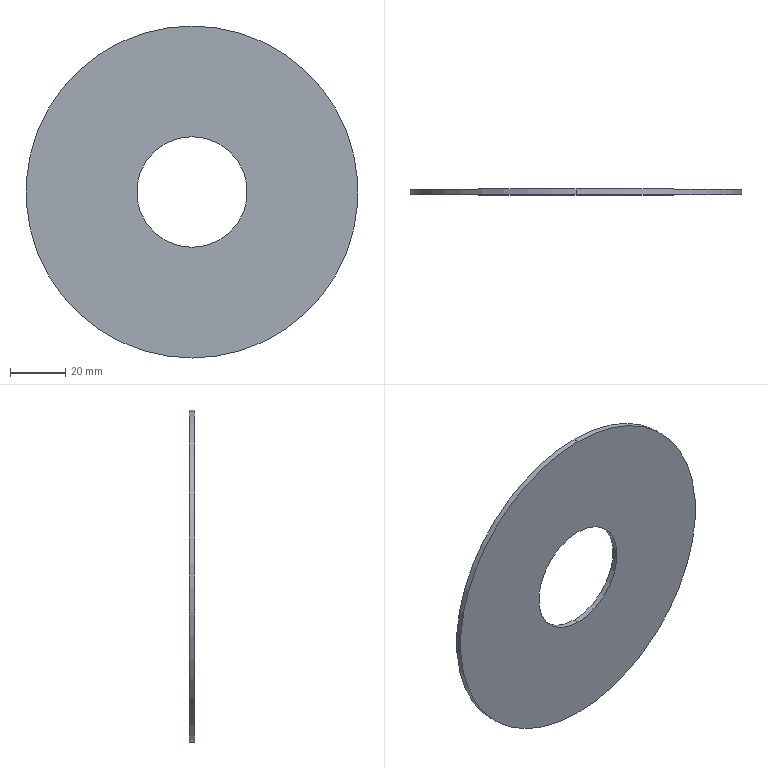Part | SolidWorks | features Extrusion 1 | 1 solid | 6 faces | box 120 x 2 x 120 mm | volume 20106 mm3 | cylinder 4 | plane 2 | commonest cylinder face diameters 40 x2 120 x2
STEP:
#1=CARTESIAN_POINT('',(0.,2.,-20.));
#2=VERTEX_POINT('',#1);
#3=CARTESIAN_POINT('',(0.,2.,20.));
#4=VERTEX_POINT('',#3);
#5=CARTESIAN_POINT('',(0.,2.,0.));
#6=DIRECTION('',(0.,1.,0.));
#7=DIRECTION('',(0.,0.,1.));
#8=AXIS2_PLACEMENT_3D('',#5,#6,#7);
#9=CIRCLE('',#8,20.);
#10=EDGE_CURVE('',#2,#4,#9,.T.);
#11=ORIENTED_EDGE('',*,*,#10,.T.);
#12=CARTESIAN_POINT('',(0.,0.,20.));
#13=VERTEX_POINT('',#12);
#14=CARTESIAN_POINT('',(0.,2.,20.));
#15=DIRECTION('',(0.,-1.,0.));
#16=VECTOR('',#15,1000.);
#17=LINE('',#14,#16);
#18=EDGE_CURVE('',#4,#13,#17,.T.);
#19=ORIENTED_EDGE('',*,*,#18,.T.);
#20=CARTESIAN_POINT('',(0.,0.,-20.));
#21=VERTEX_POINT('',#20);
#22=CARTESIAN_POINT('',(0.,0.,0.));
#23=DIRECTION('',(0.,1.,0.));
#24=DIRECTION('',(0.,0.,1.));
#25=AXIS2_PLACEMENT_3D('',#22,#23,#24);
#26=CIRCLE('',#25,20.);
#27=EDGE_CURVE('',#21,#13,#26,.T.);
#28=ORIENTED_EDGE('',*,*,#27,.F.);
#29=CARTESIAN_POINT('',(0.,2.,-20.));
#30=DIRECTION('',(0.,-1.,0.));
#31=VECTOR('',#30,1000.);
#32=LINE('',#29,#31);
#33=EDGE_CURVE('',#2,#21,#32,.T.);
#34=ORIENTED_EDGE('',*,*,#33,.F.);
#35=EDGE_LOOP('',(#11,#19,#28,#34));
#36=FACE_OUTER_BOUND('',#35,.T.);
#37=CARTESIAN_POINT('',(0.,2.,0.));
#38=DIRECTION('',(0.,-1.,0.));
#39=DIRECTION('',(0.,0.,-1.));
#40=AXIS2_PLACEMENT_3D('',#37,#38,#39);
#41=CYLINDRICAL_SURFACE('',#40,20.);
#42=ADVANCED_FACE('',(#36),#41,.F.);
#43=CARTESIAN_POINT('',(0.,2.,60.));
#44=VERTEX_POINT('',#43);
#45=CARTESIAN_POINT('',(0.,2.,-60.));
#46=VERTEX_POINT('',#45);
#47=CARTESIAN_POINT('',(0.,2.,0.));
#48=DIRECTION('',(0.,1.,0.));
#49=DIRECTION('',(0.,0.,1.));
#50=AXIS2_PLACEMENT_3D('',#47,#48,#49);
#51=CIRCLE('',#50,60.);
#52=EDGE_CURVE('',#44,#46,#51,.T.);
#53=ORIENTED_EDGE('',*,*,#52,.F.);
#54=CARTESIAN_POINT('',(0.,0.,60.));
#55=VERTEX_POINT('',#54);
#56=CARTESIAN_POINT('',(0.,2.,60.));
#57=DIRECTION('',(0.,-1.,0.));
#58=VECTOR('',#57,1000.);
#59=LINE('',#56,#58);
#60=EDGE_CURVE('',#44,#55,#59,.T.);
#61=ORIENTED_EDGE('',*,*,#60,.T.);
#62=CARTESIAN_POINT('',(0.,0.,-60.));
#63=VERTEX_POINT('',#62);
#64=CARTESIAN_POINT('',(0.,0.,0.));
#65=DIRECTION('',(0.,1.,0.));
#66=DIRECTION('',(0.,0.,1.));
#67=AXIS2_PLACEMENT_3D('',#64,#65,#66);
#68=CIRCLE('',#67,60.);
#69=EDGE_CURVE('',#55,#63,#68,.T.);
#70=ORIENTED_EDGE('',*,*,#69,.T.);
#71=CARTESIAN_POINT('',(0.,2.,-60.));
#72=DIRECTION('',(0.,-1.,0.));
#73=VECTOR('',#72,1000.);
#74=LINE('',#71,#73);
#75=EDGE_CURVE('',#46,#63,#74,.T.);
#76=ORIENTED_EDGE('',*,*,#75,.F.);
#77=EDGE_LOOP('',(#53,#61,#70,#76));
#78=FACE_OUTER_BOUND('',#77,.T.);
#79=CARTESIAN_POINT('',(0.,2.,0.));
#80=DIRECTION('',(0.,-1.,0.));
#81=DIRECTION('',(0.,0.,-1.));
#82=AXIS2_PLACEMENT_3D('',#79,#80,#81);
#83=CYLINDRICAL_SURFACE('',#82,60.);
#84=ADVANCED_FACE('',(#78),#83,.T.);
#85=CARTESIAN_POINT('',(0.,2.,0.));
#86=DIRECTION('',(0.,1.,0.));
#87=DIRECTION('',(0.,0.,1.));
#88=AXIS2_PLACEMENT_3D('',#85,#86,#87);
#89=CIRCLE('',#88,60.);
#90=EDGE_CURVE('',#46,#44,#89,.T.);
#91=ORIENTED_EDGE('',*,*,#90,.T.);
#92=ORIENTED_EDGE('',*,*,#52,.T.);
#93=EDGE_LOOP('',(#91,#92));
#94=FACE_OUTER_BOUND('',#93,.T.);
#95=ORIENTED_EDGE('',*,*,#10,.F.);
#96=CARTESIAN_POINT('',(0.,2.,0.));
#97=DIRECTION('',(0.,1.,0.));
#98=DIRECTION('',(0.,0.,1.));
#99=AXIS2_PLACEMENT_3D('',#96,#97,#98);
#100=CIRCLE('',#99,20.);
#101=EDGE_CURVE('',#4,#2,#100,.T.);
#102=ORIENTED_EDGE('',*,*,#101,.F.);
#103=EDGE_LOOP('',(#95,#102));
#104=FACE_BOUND('',#103,.T.);
#105=CARTESIAN_POINT('',(0.,2.,0.));
#106=DIRECTION('',(0.,1.,0.));
#107=DIRECTION('',(0.,0.,1.));
#108=AXIS2_PLACEMENT_3D('',#105,#106,#107);
#109=PLANE('',#108);
#110=ADVANCED_FACE('',(#94,#104),#109,.T.);
#111=CARTESIAN_POINT('',(0.,0.,0.));
#112=DIRECTION('',(0.,1.,0.));
#113=DIRECTION('',(0.,0.,1.));
#114=AXIS2_PLACEMENT_3D('',#111,#112,#113);
#115=CIRCLE('',#114,60.);
#116=EDGE_CURVE('',#63,#55,#115,.T.);
#117=ORIENTED_EDGE('',*,*,#116,.F.);
#118=ORIENTED_EDGE('',*,*,#69,.F.);
#119=EDGE_LOOP('',(#117,#118));
#120=FACE_OUTER_BOUND('',#119,.T.);
#121=ORIENTED_EDGE('',*,*,#27,.T.);
#122=CARTESIAN_POINT('',(0.,0.,0.));
#123=DIRECTION('',(0.,1.,0.));
#124=DIRECTION('',(0.,0.,1.));
#125=AXIS2_PLACEMENT_3D('',#122,#123,#124);
#126=CIRCLE('',#125,20.);
#127=EDGE_CURVE('',#13,#21,#126,.T.);
#128=ORIENTED_EDGE('',*,*,#127,.T.);
#129=EDGE_LOOP('',(#121,#128));
#130=FACE_BOUND('',#129,.T.);
#131=CARTESIAN_POINT('',(0.,0.,0.));
#132=DIRECTION('',(0.,1.,0.));
#133=DIRECTION('',(0.,0.,1.));
#134=AXIS2_PLACEMENT_3D('',#131,#132,#133);
#135=PLANE('',#134);
#136=ADVANCED_FACE('',(#120,#130),#135,.F.);
#137=ORIENTED_EDGE('',*,*,#60,.F.);
#138=ORIENTED_EDGE('',*,*,#90,.F.);
#139=ORIENTED_EDGE('',*,*,#75,.T.);
#140=ORIENTED_EDGE('',*,*,#116,.T.);
#141=EDGE_LOOP('',(#137,#138,#139,#140));
#142=FACE_OUTER_BOUND('',#141,.T.);
#143=CARTESIAN_POINT('',(0.,2.,0.));
#144=DIRECTION('',(0.,-1.,0.));
#145=DIRECTION('',(0.,0.,-1.));
#146=AXIS2_PLACEMENT_3D('',#143,#144,#145);
#147=CYLINDRICAL_SURFACE('',#146,60.);
#148=ADVANCED_FACE('',(#142),#147,.T.);
#149=ORIENTED_EDGE('',*,*,#18,.F.);
#150=ORIENTED_EDGE('',*,*,#101,.T.);
#151=ORIENTED_EDGE('',*,*,#33,.T.);
#152=ORIENTED_EDGE('',*,*,#127,.F.);
#153=EDGE_LOOP('',(#149,#150,#151,#152));
#154=FACE_OUTER_BOUND('',#153,.T.);
#155=CARTESIAN_POINT('',(0.,2.,0.));
#156=DIRECTION('',(0.,-1.,0.));
#157=DIRECTION('',(0.,0.,-1.));
#158=AXIS2_PLACEMENT_3D('',#155,#156,#157);
#159=CYLINDRICAL_SURFACE('',#158,20.);
#160=ADVANCED_FACE('',(#154),#159,.F.);
#161=CLOSED_SHELL('',(#42,#84,#110,#136,#148,#160));
#162=MANIFOLD_SOLID_BREP('',#161);
#163=CARTESIAN_POINT('',(0.,0.,0.));
#164=DIRECTION('',(0.,0.,1.));
#165=DIRECTION('',(1.,0.,0.));
#166=AXIS2_PLACEMENT_3D('',#163,#164,#165);
#167=(LENGTH_UNIT()NAMED_UNIT(*)SI_UNIT(.MILLI.,.METRE.));
#168=UNCERTAINTY_MEASURE_WITH_UNIT(LENGTH_MEASURE(0.00001),#167,'','');
#169=(NAMED_UNIT(*)PLANE_ANGLE_UNIT()SI_UNIT($,.RADIAN.));
#170=(NAMED_UNIT(*)SI_UNIT($,.STERADIAN.)SOLID_ANGLE_UNIT());
#171=(GEOMETRIC_REPRESENTATION_CONTEXT(3)GLOBAL_UNCERTAINTY_ASSIGNED_CONTEXT((#168))GLOBAL_UNIT_ASSIGNED_CONTEXT((#167,#169,#170))REPRESENTATION_CONTEXT('',''));
#172=ADVANCED_BREP_SHAPE_REPRESENTATION('',(#162,#166),#171);